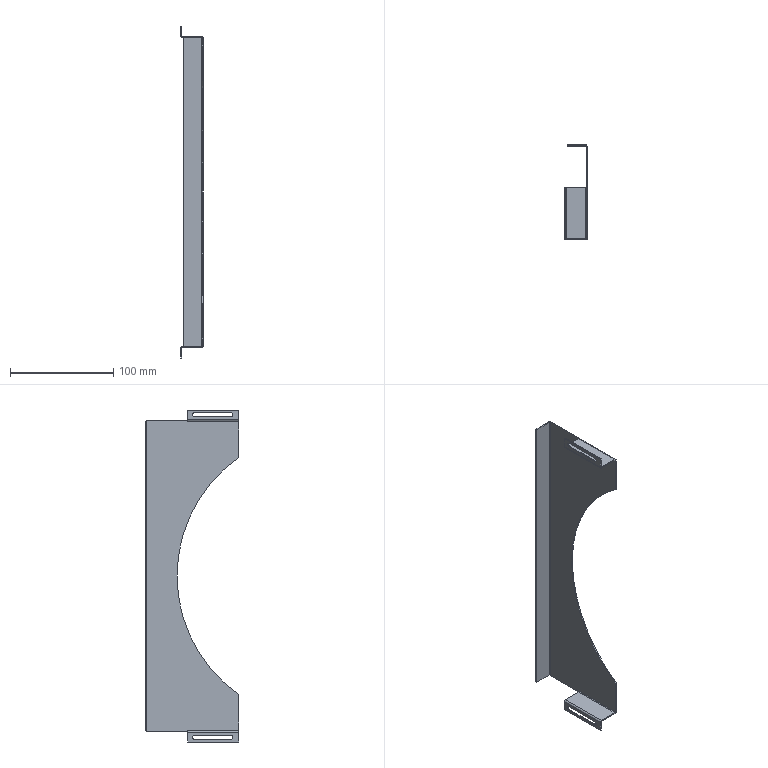Part | SolidWorks | features ICE 3, EdgeFlange 2, FlatPattern 1, SMBaseFlange 1, SheetMetal 1 | 1 solid | 61 faces | box 21.5 x 91 x 322 mm | volume 25667 mm3 | plane 43 | cylinder 18 | commonest cylinder face diameters 4 x6 1 x5 3 x5 280 x2